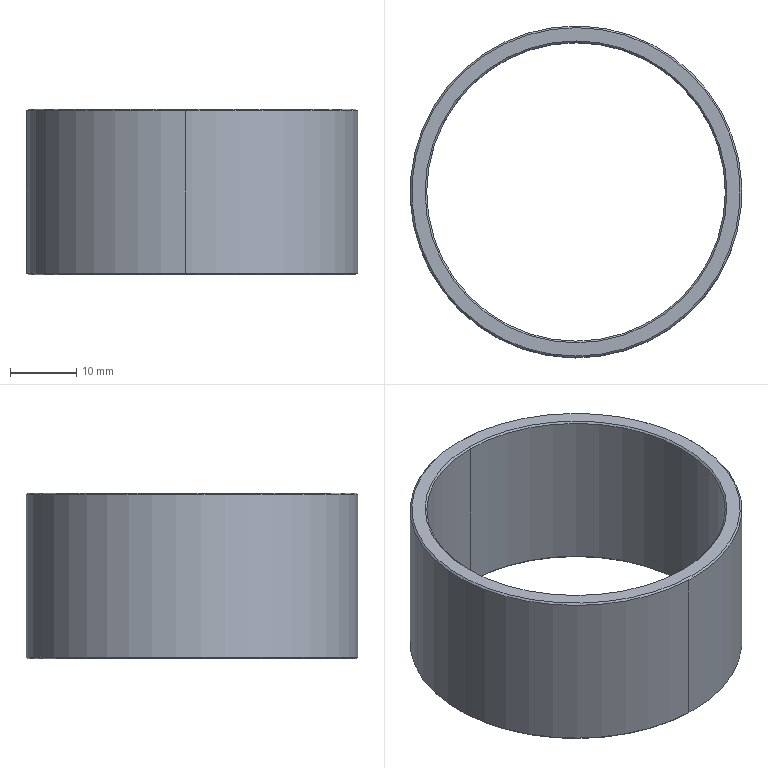Part | STEP file | 2026.6.15-Main Assembly图.sldasm-Part-149 | 1 solid | 14 faces | box 50 x 50 x 25 mm | volume 9308 mm3 | cone 8 | cylinder 4 | plane 2 | commonest cylinder face diameters 45 x2 50 x2
STEP:
#1=CARTESIAN_POINT('',(-1571.234,1449.006,3641.571));
#2=VERTEX_POINT('',#1);
#3=CARTESIAN_POINT('',(-1571.272,1399.506,3641.571));
#4=VERTEX_POINT('',#3);
#5=CARTESIAN_POINT('',(-1571.253,1424.256,3641.571));
#6=DIRECTION('',(0.,0.,-1.));
#7=DIRECTION('',(0.0007664,1.,0.));
#8=AXIS2_PLACEMENT_3D('',#5,#6,#7);
#9=CIRCLE('',#8,24.75);
#10=EDGE_CURVE('',#2,#4,#9,.T.);
#11=ORIENTED_EDGE('',*,*,#10,.F.);
#12=CARTESIAN_POINT('',(-1571.234,1449.256,3641.821));
#13=VERTEX_POINT('',#12);
#14=CARTESIAN_POINT('',(-1571.234,1449.256,3641.821));
#15=DIRECTION('',(0.000542,0.7071,0.7071));
#16=VECTOR('',#15,1000.);
#17=LINE('',#14,#16);
#18=EDGE_CURVE('',#2,#13,#17,.T.);
#19=ORIENTED_EDGE('',*,*,#18,.T.);
#20=CARTESIAN_POINT('',(-1570.28,1449.237,3641.821));
#21=VERTEX_POINT('',#20);
#22=CARTESIAN_POINT('',(-1571.253,1424.256,3641.821));
#23=DIRECTION('',(0.,0.,1.));
#24=DIRECTION('',(0.0007664,1.,0.));
#25=AXIS2_PLACEMENT_3D('',#22,#23,#24);
#26=CIRCLE('',#25,25.);
#27=EDGE_CURVE('',#21,#13,#26,.T.);
#28=ORIENTED_EDGE('',*,*,#27,.F.);
#29=CARTESIAN_POINT('',(-1571.272,1399.256,3641.821));
#30=VERTEX_POINT('',#29);
#31=CARTESIAN_POINT('',(-1571.253,1424.256,3641.821));
#32=DIRECTION('',(0.,0.,1.));
#33=DIRECTION('',(0.0007664,1.,0.));
#34=AXIS2_PLACEMENT_3D('',#31,#32,#33);
#35=CIRCLE('',#34,25.);
#36=EDGE_CURVE('',#30,#21,#35,.T.);
#37=ORIENTED_EDGE('',*,*,#36,.F.);
#38=CARTESIAN_POINT('',(-1571.272,1399.256,3641.821));
#39=DIRECTION('',(-0.000542,-0.7071,0.7071));
#40=VECTOR('',#39,1000.);
#41=LINE('',#38,#40);
#42=EDGE_CURVE('',#4,#30,#41,.T.);
#43=ORIENTED_EDGE('',*,*,#42,.F.);
#44=EDGE_LOOP('',(#11,#19,#28,#37,#43));
#45=FACE_OUTER_BOUND('',#44,.T.);
#46=CARTESIAN_POINT('',(-1571.253,1424.256,3641.821));
#47=DIRECTION('',(0.,0.,1.));
#48=DIRECTION('',(-0.0007664,-1.,0.));
#49=AXIS2_PLACEMENT_3D('',#46,#47,#48);
#50=CONICAL_SURFACE('',#49,25.,0.7854);
#51=ADVANCED_FACE('',(#45),#50,.T.);
#52=CARTESIAN_POINT('',(-1571.272,1399.506,3666.571));
#53=VERTEX_POINT('',#52);
#54=CARTESIAN_POINT('',(-1571.234,1449.006,3666.571));
#55=VERTEX_POINT('',#54);
#56=CARTESIAN_POINT('',(-1571.253,1424.256,3666.571));
#57=DIRECTION('',(0.,0.,1.));
#58=DIRECTION('',(-0.0007664,-1.,0.));
#59=AXIS2_PLACEMENT_3D('',#56,#57,#58);
#60=CIRCLE('',#59,24.75);
#61=EDGE_CURVE('',#53,#55,#60,.T.);
#62=ORIENTED_EDGE('',*,*,#61,.F.);
#63=CARTESIAN_POINT('',(-1571.272,1399.256,3666.321));
#64=VERTEX_POINT('',#63);
#65=CARTESIAN_POINT('',(-1571.272,1399.256,3666.321));
#66=DIRECTION('',(-0.000542,-0.7071,-0.7071));
#67=VECTOR('',#66,1000.);
#68=LINE('',#65,#67);
#69=EDGE_CURVE('',#53,#64,#68,.T.);
#70=ORIENTED_EDGE('',*,*,#69,.T.);
#71=CARTESIAN_POINT('',(-1570.28,1449.237,3666.321));
#72=VERTEX_POINT('',#71);
#73=CARTESIAN_POINT('',(-1571.253,1424.256,3666.321));
#74=DIRECTION('',(0.,0.,-1.));
#75=DIRECTION('',(-0.0007664,-1.,0.));
#76=AXIS2_PLACEMENT_3D('',#73,#74,#75);
#77=CIRCLE('',#76,25.);
#78=EDGE_CURVE('',#72,#64,#77,.T.);
#79=ORIENTED_EDGE('',*,*,#78,.F.);
#80=CARTESIAN_POINT('',(-1571.234,1449.256,3666.321));
#81=VERTEX_POINT('',#80);
#82=CARTESIAN_POINT('',(-1571.253,1424.256,3666.321));
#83=DIRECTION('',(0.,0.,-1.));
#84=DIRECTION('',(-0.0007664,-1.,0.));
#85=AXIS2_PLACEMENT_3D('',#82,#83,#84);
#86=CIRCLE('',#85,25.);
#87=EDGE_CURVE('',#81,#72,#86,.T.);
#88=ORIENTED_EDGE('',*,*,#87,.F.);
#89=CARTESIAN_POINT('',(-1571.234,1449.256,3666.321));
#90=DIRECTION('',(0.000542,0.7071,-0.7071));
#91=VECTOR('',#90,1000.);
#92=LINE('',#89,#91);
#93=EDGE_CURVE('',#55,#81,#92,.T.);
#94=ORIENTED_EDGE('',*,*,#93,.F.);
#95=EDGE_LOOP('',(#62,#70,#79,#88,#94));
#96=FACE_OUTER_BOUND('',#95,.T.);
#97=CARTESIAN_POINT('',(-1571.253,1424.256,3666.321));
#98=DIRECTION('',(0.,0.,-1.));
#99=DIRECTION('',(0.0007664,1.,0.));
#100=AXIS2_PLACEMENT_3D('',#97,#98,#99);
#101=CONICAL_SURFACE('',#100,25.,0.7854);
#102=ADVANCED_FACE('',(#96),#101,.T.);
#103=CARTESIAN_POINT('',(-1571.236,1446.756,3666.321));
#104=VERTEX_POINT('',#103);
#105=CARTESIAN_POINT('',(-1571.27,1401.756,3666.321));
#106=VERTEX_POINT('',#105);
#107=CARTESIAN_POINT('',(-1571.253,1424.256,3666.321));
#108=DIRECTION('',(0.,0.,1.));
#109=DIRECTION('',(-0.0007664,-1.,0.));
#110=AXIS2_PLACEMENT_3D('',#107,#108,#109);
#111=CIRCLE('',#110,22.5);
#112=EDGE_CURVE('',#104,#106,#111,.T.);
#113=ORIENTED_EDGE('',*,*,#112,.F.);
#114=CARTESIAN_POINT('',(-1571.236,1447.006,3666.571));
#115=VERTEX_POINT('',#114);
#116=CARTESIAN_POINT('',(-1571.236,1446.756,3666.321));
#117=DIRECTION('',(0.000542,0.7071,0.7071));
#118=VECTOR('',#117,1000.);
#119=LINE('',#116,#118);
#120=EDGE_CURVE('',#104,#115,#119,.T.);
#121=ORIENTED_EDGE('',*,*,#120,.T.);
#122=CARTESIAN_POINT('',(-1571.271,1401.506,3666.571));
#123=VERTEX_POINT('',#122);
#124=CARTESIAN_POINT('',(-1571.253,1424.256,3666.571));
#125=DIRECTION('',(0.,0.,-1.));
#126=DIRECTION('',(-0.0007664,-1.,0.));
#127=AXIS2_PLACEMENT_3D('',#124,#125,#126);
#128=CIRCLE('',#127,22.75);
#129=EDGE_CURVE('',#123,#115,#128,.T.);
#130=ORIENTED_EDGE('',*,*,#129,.F.);
#131=CARTESIAN_POINT('',(-1571.27,1401.756,3666.321));
#132=DIRECTION('',(-0.000542,-0.7071,0.7071));
#133=VECTOR('',#132,1000.);
#134=LINE('',#131,#133);
#135=EDGE_CURVE('',#106,#123,#134,.T.);
#136=ORIENTED_EDGE('',*,*,#135,.F.);
#137=EDGE_LOOP('',(#113,#121,#130,#136));
#138=FACE_OUTER_BOUND('',#137,.T.);
#139=CARTESIAN_POINT('',(-1571.253,1424.256,3666.321));
#140=DIRECTION('',(0.,0.,1.));
#141=DIRECTION('',(-0.0007664,-1.,0.));
#142=AXIS2_PLACEMENT_3D('',#139,#140,#141);
#143=CONICAL_SURFACE('',#142,22.5,0.7854);
#144=ADVANCED_FACE('',(#138),#143,.F.);
#145=CARTESIAN_POINT('',(-1571.27,1401.756,3641.821));
#146=VERTEX_POINT('',#145);
#147=CARTESIAN_POINT('',(-1571.236,1446.756,3641.821));
#148=VERTEX_POINT('',#147);
#149=CARTESIAN_POINT('',(-1571.253,1424.256,3641.821));
#150=DIRECTION('',(0.,0.,-1.));
#151=DIRECTION('',(0.0007664,1.,0.));
#152=AXIS2_PLACEMENT_3D('',#149,#150,#151);
#153=CIRCLE('',#152,22.5);
#154=EDGE_CURVE('',#146,#148,#153,.T.);
#155=ORIENTED_EDGE('',*,*,#154,.F.);
#156=CARTESIAN_POINT('',(-1571.271,1401.506,3641.571));
#157=VERTEX_POINT('',#156);
#158=CARTESIAN_POINT('',(-1571.271,1401.506,3641.571));
#159=DIRECTION('',(-0.000542,-0.7071,-0.7071));
#160=VECTOR('',#159,1000.);
#161=LINE('',#158,#160);
#162=EDGE_CURVE('',#146,#157,#161,.T.);
#163=ORIENTED_EDGE('',*,*,#162,.T.);
#164=CARTESIAN_POINT('',(-1571.236,1447.006,3641.571));
#165=VERTEX_POINT('',#164);
#166=CARTESIAN_POINT('',(-1571.253,1424.256,3641.571));
#167=DIRECTION('',(0.,0.,1.));
#168=DIRECTION('',(0.0007664,1.,0.));
#169=AXIS2_PLACEMENT_3D('',#166,#167,#168);
#170=CIRCLE('',#169,22.75);
#171=EDGE_CURVE('',#165,#157,#170,.T.);
#172=ORIENTED_EDGE('',*,*,#171,.F.);
#173=CARTESIAN_POINT('',(-1571.236,1447.006,3641.571));
#174=DIRECTION('',(0.000542,0.7071,-0.7071));
#175=VECTOR('',#174,1000.);
#176=LINE('',#173,#175);
#177=EDGE_CURVE('',#148,#165,#176,.T.);
#178=ORIENTED_EDGE('',*,*,#177,.F.);
#179=EDGE_LOOP('',(#155,#163,#172,#178));
#180=FACE_OUTER_BOUND('',#179,.T.);
#181=CARTESIAN_POINT('',(-1571.253,1424.256,3641.571));
#182=DIRECTION('',(0.,0.,-1.));
#183=DIRECTION('',(0.0007664,1.,0.));
#184=AXIS2_PLACEMENT_3D('',#181,#182,#183);
#185=CONICAL_SURFACE('',#184,22.75,0.7854);
#186=ADVANCED_FACE('',(#180),#185,.F.);
#187=ORIENTED_EDGE('',*,*,#154,.T.);
#188=CARTESIAN_POINT('',(-1571.236,1446.756,3641.571));
#189=DIRECTION('',(0.,0.,1.));
#190=VECTOR('',#189,1000.);
#191=LINE('',#188,#190);
#192=EDGE_CURVE('',#148,#104,#191,.T.);
#193=ORIENTED_EDGE('',*,*,#192,.T.);
#194=ORIENTED_EDGE('',*,*,#112,.T.);
#195=CARTESIAN_POINT('',(-1571.27,1401.756,3641.571));
#196=DIRECTION('',(0.,0.,1.));
#197=VECTOR('',#196,1000.);
#198=LINE('',#195,#197);
#199=EDGE_CURVE('',#146,#106,#198,.T.);
#200=ORIENTED_EDGE('',*,*,#199,.F.);
#201=EDGE_LOOP('',(#187,#193,#194,#200));
#202=FACE_OUTER_BOUND('',#201,.T.);
#203=CARTESIAN_POINT('',(-1571.253,1424.256,3641.571));
#204=DIRECTION('',(0.,0.,1.));
#205=DIRECTION('',(-0.0007664,-1.,0.));
#206=AXIS2_PLACEMENT_3D('',#203,#204,#205);
#207=CYLINDRICAL_SURFACE('',#206,22.5);
#208=ADVANCED_FACE('',(#202),#207,.F.);
#209=ORIENTED_EDGE('',*,*,#78,.T.);
#210=CARTESIAN_POINT('',(-1572.226,1399.275,3666.321));
#211=VERTEX_POINT('',#210);
#212=CARTESIAN_POINT('',(-1571.253,1424.256,3666.321));
#213=DIRECTION('',(0.,0.,-1.));
#214=DIRECTION('',(-0.0007664,-1.,0.));
#215=AXIS2_PLACEMENT_3D('',#212,#213,#214);
#216=CIRCLE('',#215,25.);
#217=EDGE_CURVE('',#64,#211,#216,.T.);
#218=ORIENTED_EDGE('',*,*,#217,.T.);
#219=CARTESIAN_POINT('',(-1572.226,1399.275,3641.821));
#220=VERTEX_POINT('',#219);
#221=CARTESIAN_POINT('',(-1572.226,1399.275,3666.571));
#222=DIRECTION('',(0.,0.,-1.));
#223=VECTOR('',#222,1000.);
#224=LINE('',#221,#223);
#225=EDGE_CURVE('',#211,#220,#224,.T.);
#226=ORIENTED_EDGE('',*,*,#225,.T.);
#227=CARTESIAN_POINT('',(-1571.253,1424.256,3641.821));
#228=DIRECTION('',(0.,0.,1.));
#229=DIRECTION('',(0.0007664,1.,0.));
#230=AXIS2_PLACEMENT_3D('',#227,#228,#229);
#231=CIRCLE('',#230,25.);
#232=EDGE_CURVE('',#220,#30,#231,.T.);
#233=ORIENTED_EDGE('',*,*,#232,.T.);
#234=ORIENTED_EDGE('',*,*,#36,.T.);
#235=CARTESIAN_POINT('',(-1570.28,1449.237,3666.571));
#236=DIRECTION('',(0.,0.,-1.));
#237=VECTOR('',#236,1000.);
#238=LINE('',#235,#237);
#239=EDGE_CURVE('',#72,#21,#238,.T.);
#240=ORIENTED_EDGE('',*,*,#239,.F.);
#241=EDGE_LOOP('',(#209,#218,#226,#233,#234,#240));
#242=FACE_OUTER_BOUND('',#241,.T.);
#243=CARTESIAN_POINT('',(-1571.253,1424.256,3666.571));
#244=DIRECTION('',(0.,0.,-1.));
#245=DIRECTION('',(0.03892,0.9992,0.));
#246=AXIS2_PLACEMENT_3D('',#243,#244,#245);
#247=CYLINDRICAL_SURFACE('',#246,25.);
#248=ADVANCED_FACE('',(#242),#247,.T.);
#249=ORIENTED_EDGE('',*,*,#171,.T.);
#250=CARTESIAN_POINT('',(-1571.253,1424.256,3641.571));
#251=DIRECTION('',(0.,0.,1.));
#252=DIRECTION('',(0.0007664,1.,0.));
#253=AXIS2_PLACEMENT_3D('',#250,#251,#252);
#254=CIRCLE('',#253,22.75);
#255=EDGE_CURVE('',#157,#165,#254,.T.);
#256=ORIENTED_EDGE('',*,*,#255,.T.);
#257=EDGE_LOOP('',(#249,#256));
#258=FACE_BOUND('',#257,.T.);
#259=CARTESIAN_POINT('',(-1571.253,1424.256,3641.571));
#260=DIRECTION('',(0.,0.,-1.));
#261=DIRECTION('',(0.0007664,1.,0.));
#262=AXIS2_PLACEMENT_3D('',#259,#260,#261);
#263=CIRCLE('',#262,24.75);
#264=EDGE_CURVE('',#4,#2,#263,.T.);
#265=ORIENTED_EDGE('',*,*,#264,.T.);
#266=ORIENTED_EDGE('',*,*,#10,.T.);
#267=EDGE_LOOP('',(#265,#266));
#268=FACE_OUTER_BOUND('',#267,.T.);
#269=CARTESIAN_POINT('',(-1571.253,1424.256,3641.571));
#270=DIRECTION('',(0.,0.,-1.));
#271=DIRECTION('',(0.0007664,1.,0.));
#272=AXIS2_PLACEMENT_3D('',#269,#270,#271);
#273=PLANE('',#272);
#274=ADVANCED_FACE('',(#258,#268),#273,.T.);
#275=ORIENTED_EDGE('',*,*,#129,.T.);
#276=CARTESIAN_POINT('',(-1571.253,1424.256,3666.571));
#277=DIRECTION('',(0.,0.,-1.));
#278=DIRECTION('',(-0.0007664,-1.,0.));
#279=AXIS2_PLACEMENT_3D('',#276,#277,#278);
#280=CIRCLE('',#279,22.75);
#281=EDGE_CURVE('',#115,#123,#280,.T.);
#282=ORIENTED_EDGE('',*,*,#281,.T.);
#283=EDGE_LOOP('',(#275,#282));
#284=FACE_BOUND('',#283,.T.);
#285=CARTESIAN_POINT('',(-1571.253,1424.256,3666.571));
#286=DIRECTION('',(0.,0.,1.));
#287=DIRECTION('',(-0.0007664,-1.,0.));
#288=AXIS2_PLACEMENT_3D('',#285,#286,#287);
#289=CIRCLE('',#288,24.75);
#290=EDGE_CURVE('',#55,#53,#289,.T.);
#291=ORIENTED_EDGE('',*,*,#290,.T.);
#292=ORIENTED_EDGE('',*,*,#61,.T.);
#293=EDGE_LOOP('',(#291,#292));
#294=FACE_OUTER_BOUND('',#293,.T.);
#295=CARTESIAN_POINT('',(-1571.253,1424.256,3666.571));
#296=DIRECTION('',(0.,0.,1.));
#297=DIRECTION('',(-0.0007664,-1.,0.));
#298=AXIS2_PLACEMENT_3D('',#295,#296,#297);
#299=PLANE('',#298);
#300=ADVANCED_FACE('',(#284,#294),#299,.T.);
#301=ORIENTED_EDGE('',*,*,#225,.F.);
#302=CARTESIAN_POINT('',(-1571.253,1424.256,3666.321));
#303=DIRECTION('',(0.,0.,-1.));
#304=DIRECTION('',(-0.0007664,-1.,0.));
#305=AXIS2_PLACEMENT_3D('',#302,#303,#304);
#306=CIRCLE('',#305,25.);
#307=EDGE_CURVE('',#211,#81,#306,.T.);
#308=ORIENTED_EDGE('',*,*,#307,.T.);
#309=ORIENTED_EDGE('',*,*,#87,.T.);
#310=ORIENTED_EDGE('',*,*,#239,.T.);
#311=ORIENTED_EDGE('',*,*,#27,.T.);
#312=CARTESIAN_POINT('',(-1571.253,1424.256,3641.821));
#313=DIRECTION('',(0.,0.,1.));
#314=DIRECTION('',(0.0007664,1.,0.));
#315=AXIS2_PLACEMENT_3D('',#312,#313,#314);
#316=CIRCLE('',#315,25.);
#317=EDGE_CURVE('',#13,#220,#316,.T.);
#318=ORIENTED_EDGE('',*,*,#317,.T.);
#319=EDGE_LOOP('',(#301,#308,#309,#310,#311,#318));
#320=FACE_OUTER_BOUND('',#319,.T.);
#321=CARTESIAN_POINT('',(-1571.253,1424.256,3666.571));
#322=DIRECTION('',(0.,0.,-1.));
#323=DIRECTION('',(0.03892,0.9992,0.));
#324=AXIS2_PLACEMENT_3D('',#321,#322,#323);
#325=CYLINDRICAL_SURFACE('',#324,25.);
#326=ADVANCED_FACE('',(#320),#325,.T.);
#327=ORIENTED_EDGE('',*,*,#192,.F.);
#328=CARTESIAN_POINT('',(-1571.253,1424.256,3641.821));
#329=DIRECTION('',(0.,0.,-1.));
#330=DIRECTION('',(0.0007664,1.,0.));
#331=AXIS2_PLACEMENT_3D('',#328,#329,#330);
#332=CIRCLE('',#331,22.5);
#333=EDGE_CURVE('',#148,#146,#332,.T.);
#334=ORIENTED_EDGE('',*,*,#333,.T.);
#335=ORIENTED_EDGE('',*,*,#199,.T.);
#336=CARTESIAN_POINT('',(-1571.253,1424.256,3666.321));
#337=DIRECTION('',(0.,0.,1.));
#338=DIRECTION('',(-0.0007664,-1.,0.));
#339=AXIS2_PLACEMENT_3D('',#336,#337,#338);
#340=CIRCLE('',#339,22.5);
#341=EDGE_CURVE('',#106,#104,#340,.T.);
#342=ORIENTED_EDGE('',*,*,#341,.T.);
#343=EDGE_LOOP('',(#327,#334,#335,#342));
#344=FACE_OUTER_BOUND('',#343,.T.);
#345=CARTESIAN_POINT('',(-1571.253,1424.256,3641.571));
#346=DIRECTION('',(0.,0.,1.));
#347=DIRECTION('',(-0.0007664,-1.,0.));
#348=AXIS2_PLACEMENT_3D('',#345,#346,#347);
#349=CYLINDRICAL_SURFACE('',#348,22.5);
#350=ADVANCED_FACE('',(#344),#349,.F.);
#351=ORIENTED_EDGE('',*,*,#162,.F.);
#352=ORIENTED_EDGE('',*,*,#333,.F.);
#353=ORIENTED_EDGE('',*,*,#177,.T.);
#354=ORIENTED_EDGE('',*,*,#255,.F.);
#355=EDGE_LOOP('',(#351,#352,#353,#354));
#356=FACE_OUTER_BOUND('',#355,.T.);
#357=CARTESIAN_POINT('',(-1571.253,1424.256,3641.571));
#358=DIRECTION('',(0.,0.,-1.));
#359=DIRECTION('',(0.0007664,1.,0.));
#360=AXIS2_PLACEMENT_3D('',#357,#358,#359);
#361=CONICAL_SURFACE('',#360,22.75,0.7854);
#362=ADVANCED_FACE('',(#356),#361,.F.);
#363=ORIENTED_EDGE('',*,*,#120,.F.);
#364=ORIENTED_EDGE('',*,*,#341,.F.);
#365=ORIENTED_EDGE('',*,*,#135,.T.);
#366=ORIENTED_EDGE('',*,*,#281,.F.);
#367=EDGE_LOOP('',(#363,#364,#365,#366));
#368=FACE_OUTER_BOUND('',#367,.T.);
#369=CARTESIAN_POINT('',(-1571.253,1424.256,3666.321));
#370=DIRECTION('',(0.,0.,1.));
#371=DIRECTION('',(-0.0007664,-1.,0.));
#372=AXIS2_PLACEMENT_3D('',#369,#370,#371);
#373=CONICAL_SURFACE('',#372,22.5,0.7854);
#374=ADVANCED_FACE('',(#368),#373,.F.);
#375=ORIENTED_EDGE('',*,*,#69,.F.);
#376=ORIENTED_EDGE('',*,*,#290,.F.);
#377=ORIENTED_EDGE('',*,*,#93,.T.);
#378=ORIENTED_EDGE('',*,*,#307,.F.);
#379=ORIENTED_EDGE('',*,*,#217,.F.);
#380=EDGE_LOOP('',(#375,#376,#377,#378,#379));
#381=FACE_OUTER_BOUND('',#380,.T.);
#382=CARTESIAN_POINT('',(-1571.253,1424.256,3666.321));
#383=DIRECTION('',(0.,0.,-1.));
#384=DIRECTION('',(0.0007664,1.,0.));
#385=AXIS2_PLACEMENT_3D('',#382,#383,#384);
#386=CONICAL_SURFACE('',#385,25.,0.7854);
#387=ADVANCED_FACE('',(#381),#386,.T.);
#388=ORIENTED_EDGE('',*,*,#18,.F.);
#389=ORIENTED_EDGE('',*,*,#264,.F.);
#390=ORIENTED_EDGE('',*,*,#42,.T.);
#391=ORIENTED_EDGE('',*,*,#232,.F.);
#392=ORIENTED_EDGE('',*,*,#317,.F.);
#393=EDGE_LOOP('',(#388,#389,#390,#391,#392));
#394=FACE_OUTER_BOUND('',#393,.T.);
#395=CARTESIAN_POINT('',(-1571.253,1424.256,3641.821));
#396=DIRECTION('',(0.,0.,1.));
#397=DIRECTION('',(-0.0007664,-1.,0.));
#398=AXIS2_PLACEMENT_3D('',#395,#396,#397);
#399=CONICAL_SURFACE('',#398,25.,0.7854);
#400=ADVANCED_FACE('',(#394),#399,.T.);
#401=CLOSED_SHELL('',(#51,#102,#144,#186,#208,#248,#274,#300,#326,#350,#362,#374,#387,#400));
#402=MANIFOLD_SOLID_BREP('',#401);
#403=CARTESIAN_POINT('',(0.,0.,0.));
#404=DIRECTION('',(0.,0.,1.));
#405=DIRECTION('',(1.,0.,0.));
#406=AXIS2_PLACEMENT_3D('',#403,#404,#405);
#407=(LENGTH_UNIT()NAMED_UNIT(*)SI_UNIT(.MILLI.,.METRE.));
#408=UNCERTAINTY_MEASURE_WITH_UNIT(LENGTH_MEASURE(0.00001),#407,'','');
#409=(NAMED_UNIT(*)PLANE_ANGLE_UNIT()SI_UNIT($,.RADIAN.));
#410=(NAMED_UNIT(*)SI_UNIT($,.STERADIAN.)SOLID_ANGLE_UNIT());
#411=(GEOMETRIC_REPRESENTATION_CONTEXT(3)GLOBAL_UNCERTAINTY_ASSIGNED_CONTEXT((#408))GLOBAL_UNIT_ASSIGNED_CONTEXT((#407,#409,#410))REPRESENTATION_CONTEXT('',''));
#412=ADVANCED_BREP_SHAPE_REPRESENTATION('',(#402,#406),#411);